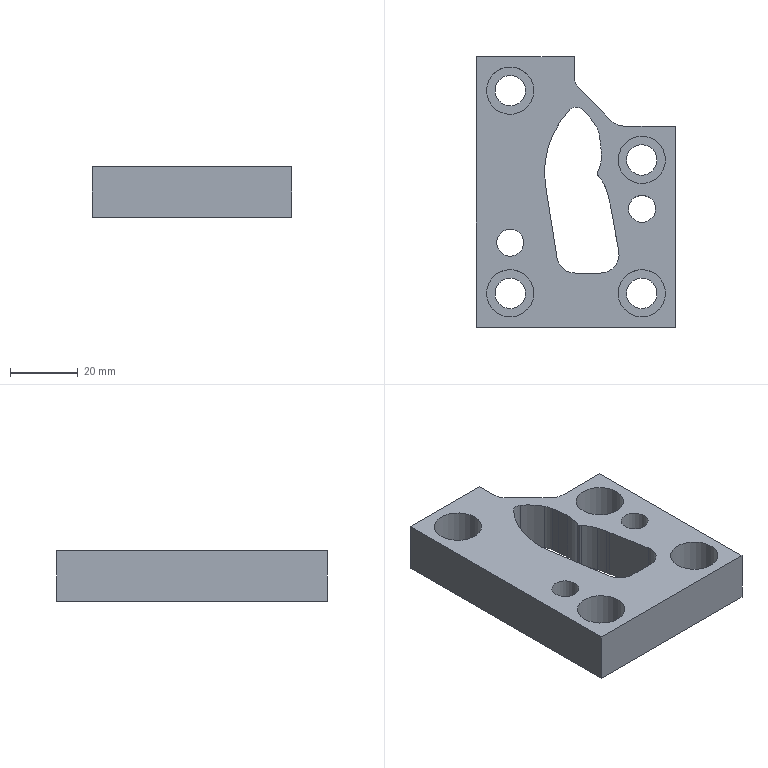Part | STEP file | 1 solid | 43 faces | box 58.914 x 80 x 15 mm | volume 42146 mm3 | cylinder 26 | plane 15 | spline 2 | commonest cylinder face diameters 9 x4 14 x4 8 x2 10 x2 11 x2 1.518 x1
STEP:
#1=CARTESIAN_POINT('',(-239.5,-87.5,-17.));
#2=VERTEX_POINT('',#1);
#3=CARTESIAN_POINT('',(-243.5,-87.5,-17.));
#4=DIRECTION('',(0.,0.,1.));
#5=DIRECTION('',(1.,0.,0.));
#6=AXIS2_PLACEMENT_3D('',#3,#4,#5);
#7=CIRCLE('',#6,4.);
#8=EDGE_CURVE('',#2,#2,#7,.T.);
#9=ORIENTED_EDGE('',*,*,#8,.T.);
#10=EDGE_LOOP('',(#9));
#11=FACE_BOUND('',#10,.T.);
#12=CARTESIAN_POINT('',(-278.5,-97.5,-17.));
#13=VERTEX_POINT('',#12);
#14=CARTESIAN_POINT('',(-282.5,-97.5,-17.));
#15=DIRECTION('',(0.,0.,1.));
#16=DIRECTION('',(1.,0.,0.));
#17=AXIS2_PLACEMENT_3D('',#14,#15,#16);
#18=CIRCLE('',#17,4.);
#19=EDGE_CURVE('',#13,#13,#18,.T.);
#20=ORIENTED_EDGE('',*,*,#19,.T.);
#21=EDGE_LOOP('',(#20));
#22=FACE_BOUND('',#21,.T.);
#23=CARTESIAN_POINT('',(-239.086,-73.,-17.));
#24=VERTEX_POINT('',#23);
#25=CARTESIAN_POINT('',(-243.586,-73.,-17.));
#26=DIRECTION('',(0.,0.,-1.));
#27=DIRECTION('',(1.,0.,0.));
#28=AXIS2_PLACEMENT_3D('',#25,#26,#27);
#29=CIRCLE('',#28,4.5);
#30=EDGE_CURVE('',#24,#24,#29,.T.);
#31=ORIENTED_EDGE('',*,*,#30,.F.);
#32=EDGE_LOOP('',(#31));
#33=FACE_BOUND('',#32,.T.);
#34=CARTESIAN_POINT('',(-287.,-112.5,-17.));
#35=VERTEX_POINT('',#34);
#36=CARTESIAN_POINT('',(-282.5,-112.5,-17.));
#37=DIRECTION('',(0.,0.,-1.));
#38=DIRECTION('',(-1.,0.,0.));
#39=AXIS2_PLACEMENT_3D('',#36,#37,#38);
#40=CIRCLE('',#39,4.5);
#41=EDGE_CURVE('',#35,#35,#40,.T.);
#42=ORIENTED_EDGE('',*,*,#41,.F.);
#43=EDGE_LOOP('',(#42));
#44=FACE_BOUND('',#43,.T.);
#45=CARTESIAN_POINT('',(-287.,-52.5,-17.));
#46=VERTEX_POINT('',#45);
#47=CARTESIAN_POINT('',(-282.5,-52.5,-17.));
#48=DIRECTION('',(0.,0.,1.));
#49=DIRECTION('',(-1.,0.,0.));
#50=AXIS2_PLACEMENT_3D('',#47,#48,#49);
#51=CIRCLE('',#50,4.5);
#52=EDGE_CURVE('',#46,#46,#51,.T.);
#53=ORIENTED_EDGE('',*,*,#52,.T.);
#54=EDGE_LOOP('',(#53));
#55=FACE_BOUND('',#54,.T.);
#56=CARTESIAN_POINT('',(-239.086,-112.5,-17.));
#57=VERTEX_POINT('',#56);
#58=CARTESIAN_POINT('',(-243.586,-112.5,-17.));
#59=DIRECTION('',(0.,0.,1.));
#60=DIRECTION('',(1.,0.,0.));
#61=AXIS2_PLACEMENT_3D('',#58,#59,#60);
#62=CIRCLE('',#61,4.5);
#63=EDGE_CURVE('',#57,#57,#62,.T.);
#64=ORIENTED_EDGE('',*,*,#63,.T.);
#65=EDGE_LOOP('',(#64));
#66=FACE_BOUND('',#65,.T.);
#67=CARTESIAN_POINT('',(-263.55,-48.378,-17.));
#68=VERTEX_POINT('',#67);
#69=CARTESIAN_POINT('',(-263.55,-42.5,-17.));
#70=VERTEX_POINT('',#69);
#71=CARTESIAN_POINT('',(-263.55,47.,-17.));
#72=DIRECTION('',(0.,1.,0.));
#73=VECTOR('',#72,1.);
#74=LINE('',#71,#73);
#75=EDGE_CURVE('',#68,#70,#74,.T.);
#76=ORIENTED_EDGE('',*,*,#75,.F.);
#77=CARTESIAN_POINT('',(-262.086,-51.914,-17.));
#78=VERTEX_POINT('',#77);
#79=CARTESIAN_POINT('',(-258.55,-48.378,-17.));
#80=DIRECTION('',(0.,0.,1.));
#81=DIRECTION('',(1.,0.,0.));
#82=AXIS2_PLACEMENT_3D('',#79,#80,#81);
#83=CIRCLE('',#82,5.);
#84=EDGE_CURVE('',#68,#78,#83,.T.);
#85=ORIENTED_EDGE('',*,*,#84,.T.);
#86=CARTESIAN_POINT('',(-252.464,-61.536,-17.));
#87=VERTEX_POINT('',#86);
#88=CARTESIAN_POINT('',(-203.505,-110.494,-17.));
#89=DIRECTION('',(0.7071,-0.7071,0.));
#90=VECTOR('',#89,1.);
#91=LINE('',#88,#90);
#92=EDGE_CURVE('',#78,#87,#91,.T.);
#93=ORIENTED_EDGE('',*,*,#92,.T.);
#94=CARTESIAN_POINT('',(-248.928,-63.,-17.));
#95=VERTEX_POINT('',#94);
#96=CARTESIAN_POINT('',(-248.928,-58.,-17.));
#97=DIRECTION('',(0.,0.,1.));
#98=DIRECTION('',(1.,0.,0.));
#99=AXIS2_PLACEMENT_3D('',#96,#97,#98);
#100=CIRCLE('',#99,5.);
#101=EDGE_CURVE('',#87,#95,#100,.T.);
#102=ORIENTED_EDGE('',*,*,#101,.T.);
#103=CARTESIAN_POINT('',(-233.586,-63.,-17.));
#104=VERTEX_POINT('',#103);
#105=CARTESIAN_POINT('',(-224.,-63.,-17.));
#106=DIRECTION('',(-1.,0.,0.));
#107=VECTOR('',#106,1.);
#108=LINE('',#105,#107);
#109=EDGE_CURVE('',#104,#95,#108,.T.);
#110=ORIENTED_EDGE('',*,*,#109,.F.);
#111=CARTESIAN_POINT('',(-233.586,-122.5,-17.));
#112=VERTEX_POINT('',#111);
#113=CARTESIAN_POINT('',(-233.586,-97.5,-17.));
#114=DIRECTION('',(0.,1.,0.));
#115=VECTOR('',#114,1.);
#116=LINE('',#113,#115);
#117=EDGE_CURVE('',#112,#104,#116,.T.);
#118=ORIENTED_EDGE('',*,*,#117,.F.);
#119=CARTESIAN_POINT('',(-292.5,-122.5,-17.));
#120=VERTEX_POINT('',#119);
#121=CARTESIAN_POINT('',(-262.5,-122.5,-17.));
#122=DIRECTION('',(1.,0.,0.));
#123=VECTOR('',#122,1.);
#124=LINE('',#121,#123);
#125=EDGE_CURVE('',#120,#112,#124,.T.);
#126=ORIENTED_EDGE('',*,*,#125,.F.);
#127=CARTESIAN_POINT('',(-292.5,-42.5,-17.));
#128=VERTEX_POINT('',#127);
#129=CARTESIAN_POINT('',(-292.5,49.2,-17.));
#130=DIRECTION('',(0.,1.,0.));
#131=VECTOR('',#130,1.);
#132=LINE('',#129,#131);
#133=EDGE_CURVE('',#120,#128,#132,.T.);
#134=ORIENTED_EDGE('',*,*,#133,.T.);
#135=CARTESIAN_POINT('',(-262.5,-42.5,-17.));
#136=DIRECTION('',(-1.,0.,0.));
#137=VECTOR('',#136,1.);
#138=LINE('',#135,#137);
#139=EDGE_CURVE('',#70,#128,#138,.T.);
#140=ORIENTED_EDGE('',*,*,#139,.F.);
#141=EDGE_LOOP('',(#76,#85,#93,#102,#110,#118,#126,#134,#140));
#142=FACE_BOUND('',#141,.T.);
#143=CARTESIAN_POINT('',(-250.392,-100.011,-17.));
#144=VERTEX_POINT('',#143);
#145=CARTESIAN_POINT('',(-255.802,-106.5,-17.));
#146=VERTEX_POINT('',#145);
#147=CARTESIAN_POINT('',(-255.802,-101.,-17.));
#148=DIRECTION('',(0.,0.,-1.));
#149=DIRECTION('',(1.,0.,0.));
#150=AXIS2_PLACEMENT_3D('',#147,#148,#149);
#151=CIRCLE('',#150,5.5);
#152=EDGE_CURVE('',#144,#146,#151,.T.);
#153=ORIENTED_EDGE('',*,*,#152,.F.);
#154=CARTESIAN_POINT('',(-252.857,-86.509,-17.));
#155=VERTEX_POINT('',#154);
#156=CARTESIAN_POINT('',(33298.208,6031.949,-17.));
#157=DIRECTION('',(0.,0.,-1.));
#158=DIRECTION('',(1.,0.,0.));
#159=AXIS2_PLACEMENT_3D('',#156,#157,#158);
#160=CIRCLE('',#159,34104.391);
#161=EDGE_CURVE('',#144,#155,#160,.T.);
#162=ORIENTED_EDGE('',*,*,#161,.T.);
#163=CARTESIAN_POINT('',(-253.088,-85.35,-17.));
#164=VERTEX_POINT('',#163);
#165=CARTESIAN_POINT('',(-289.905,-93.275,-17.));
#166=DIRECTION('',(0.,0.,1.));
#167=DIRECTION('',(1.,0.,0.));
#168=AXIS2_PLACEMENT_3D('',#165,#166,#167);
#169=CIRCLE('',#168,37.66);
#170=EDGE_CURVE('',#155,#164,#169,.T.);
#171=ORIENTED_EDGE('',*,*,#170,.T.);
#172=CARTESIAN_POINT('',(-253.879,-82.262,-17.));
#173=VERTEX_POINT('',#172);
#174=CARTESIAN_POINT('',(-292.811,-93.913,-17.));
#175=DIRECTION('',(0.,0.,1.));
#176=DIRECTION('',(1.,0.,0.));
#177=AXIS2_PLACEMENT_3D('',#174,#175,#176);
#178=CIRCLE('',#177,40.635);
#179=EDGE_CURVE('',#164,#173,#178,.T.);
#180=ORIENTED_EDGE('',*,*,#179,.T.);
#181=CARTESIAN_POINT('',(-256.293,-77.948,-17.));
#182=VERTEX_POINT('',#181);
#183=CARTESIAN_POINT('',(-264.943,-85.623,-17.));
#184=DIRECTION('',(0.,0.,1.));
#185=DIRECTION('',(1.,0.,0.));
#186=AXIS2_PLACEMENT_3D('',#183,#184,#185);
#187=CIRCLE('',#186,11.564);
#188=EDGE_CURVE('',#173,#182,#187,.T.);
#189=ORIENTED_EDGE('',*,*,#188,.T.);
#190=CARTESIAN_POINT('',(-256.599,-77.557,-17.));
#191=VERTEX_POINT('',#190);
#192=CARTESIAN_POINT('',(-252.81,-74.892,-17.));
#193=DIRECTION('',(0.,0.,-1.));
#194=DIRECTION('',(1.,0.,0.));
#195=AXIS2_PLACEMENT_3D('',#192,#193,#194);
#196=CIRCLE('',#195,4.634);
#197=EDGE_CURVE('',#182,#191,#196,.T.);
#198=ORIENTED_EDGE('',*,*,#197,.T.);
#199=CARTESIAN_POINT('',(-256.698,-76.822,-17.));
#200=VERTEX_POINT('',#199);
#201=CARTESIAN_POINT('',(-255.992,-77.101,-17.));
#202=DIRECTION('',(0.,0.,-1.));
#203=DIRECTION('',(1.,0.,0.));
#204=AXIS2_PLACEMENT_3D('',#201,#202,#203);
#205=CIRCLE('',#204,0.7592);
#206=EDGE_CURVE('',#191,#200,#205,.T.);
#207=ORIENTED_EDGE('',*,*,#206,.T.);
#208=CARTESIAN_POINT('',(-256.574,-76.515,-17.));
#209=VERTEX_POINT('',#208);
#210=CARTESIAN_POINT('',(-253.687,-77.89,-17.));
#211=DIRECTION('',(0.,0.,-1.));
#212=DIRECTION('',(1.,0.,0.));
#213=AXIS2_PLACEMENT_3D('',#210,#211,#212);
#214=CIRCLE('',#213,3.195);
#215=EDGE_CURVE('',#200,#209,#214,.T.);
#216=ORIENTED_EDGE('',*,*,#215,.T.);
#217=CARTESIAN_POINT('',(-255.525,-71.581,-17.));
#218=VERTEX_POINT('',#217);
#219=CARTESIAN_POINT('',(-266.229,-71.882,-17.));
#220=DIRECTION('',(0.,0.,1.));
#221=DIRECTION('',(1.,0.,0.));
#222=AXIS2_PLACEMENT_3D('',#219,#220,#221);
#223=CIRCLE('',#222,10.71);
#224=EDGE_CURVE('',#209,#218,#223,.T.);
#225=ORIENTED_EDGE('',*,*,#224,.T.);
#226=CARTESIAN_POINT('',(-255.83,-68.058,-17.));
#227=VERTEX_POINT('',#226);
#228=CARTESIAN_POINT('',(-288.806,-72.678,-17.));
#229=DIRECTION('',(0.,0.,1.));
#230=DIRECTION('',(1.,0.,0.));
#231=AXIS2_PLACEMENT_3D('',#228,#229,#230);
#232=CIRCLE('',#231,33.298);
#233=EDGE_CURVE('',#218,#227,#232,.T.);
#234=ORIENTED_EDGE('',*,*,#233,.T.);
#235=CARTESIAN_POINT('',(-256.146,-65.761,-17.));
#236=VERTEX_POINT('',#235);
#237=CARTESIAN_POINT('',(286.525,7.944,-17.));
#238=DIRECTION('',(0.,0.,-1.));
#239=DIRECTION('',(1.,0.,0.));
#240=AXIS2_PLACEMENT_3D('',#237,#238,#239);
#241=CIRCLE('',#240,547.653);
#242=EDGE_CURVE('',#227,#236,#241,.T.);
#243=ORIENTED_EDGE('',*,*,#242,.T.);
#244=CARTESIAN_POINT('',(-257.012,-63.252,-17.));
#245=VERTEX_POINT('',#244);
#246=CARTESIAN_POINT('',(-262.853,-66.672,-17.));
#247=DIRECTION('',(0.,0.,1.));
#248=DIRECTION('',(1.,0.,0.));
#249=AXIS2_PLACEMENT_3D('',#246,#247,#248);
#250=CIRCLE('',#249,6.768);
#251=EDGE_CURVE('',#236,#245,#250,.T.);
#252=ORIENTED_EDGE('',*,*,#251,.T.);
#253=CARTESIAN_POINT('',(-261.559,-57.918,-17.));
#254=VERTEX_POINT('',#253);
#255=CARTESIAN_POINT('',(-257.012,-63.252,-17.));
#256=CARTESIAN_POINT('',(-258.204,-61.218,-17.));
#257=CARTESIAN_POINT('',(-259.658,-59.325,-17.));
#258=CARTESIAN_POINT('',(-261.559,-57.918,-17.));
#259=B_SPLINE_CURVE_WITH_KNOTS('',3,(#255,#256,#257,#258),.UNSPECIFIED.,.F.,.F.,(4,4),(0.,1.),.UNSPECIFIED.);
#260=EDGE_CURVE('',#245,#254,#259,.T.);
#261=ORIENTED_EDGE('',*,*,#260,.T.);
#262=CARTESIAN_POINT('',(-264.842,-58.187,-17.));
#263=VERTEX_POINT('',#262);
#264=CARTESIAN_POINT('',(-263.047,-59.927,-17.));
#265=DIRECTION('',(0.,0.,-1.));
#266=DIRECTION('',(1.,0.,0.));
#267=AXIS2_PLACEMENT_3D('',#264,#265,#266);
#268=CIRCLE('',#267,2.5);
#269=EDGE_CURVE('',#263,#254,#268,.T.);
#270=ORIENTED_EDGE('',*,*,#269,.F.);
#271=CARTESIAN_POINT('',(-271.999,-80.759,-17.));
#272=VERTEX_POINT('',#271);
#273=CARTESIAN_POINT('',(-264.842,-58.187,-17.));
#274=CARTESIAN_POINT('',(-266.278,-59.668,-17.));
#275=CARTESIAN_POINT('',(-267.514,-61.287,-17.));
#276=CARTESIAN_POINT('',(-269.608,-64.784,-17.));
#277=CARTESIAN_POINT('',(-270.466,-66.681,-17.));
#278=CARTESIAN_POINT('',(-272.311,-72.501,-17.));
#279=CARTESIAN_POINT('',(-272.635,-76.684,-17.));
#280=CARTESIAN_POINT('',(-271.999,-80.759,-17.));
#281=B_SPLINE_CURVE_WITH_KNOTS('',3,(#273,#274,#275,#276,#277,#278,#279,#280),.UNSPECIFIED.,.F.,.F.,(4,2,2,4),(0.,0.25,0.5,1.),.UNSPECIFIED.);
#282=EDGE_CURVE('',#263,#272,#281,.T.);
#283=ORIENTED_EDGE('',*,*,#282,.T.);
#284=CARTESIAN_POINT('',(-268.678,-101.855,-17.));
#285=VERTEX_POINT('',#284);
#286=CARTESIAN_POINT('',(-286.444,11.004,-17.));
#287=DIRECTION('',(0.1555,-0.9878,0.));
#288=VECTOR('',#287,1.);
#289=LINE('',#286,#288);
#290=EDGE_CURVE('',#272,#285,#289,.T.);
#291=ORIENTED_EDGE('',*,*,#290,.T.);
#292=CARTESIAN_POINT('',(-263.245,-106.5,-17.));
#293=VERTEX_POINT('',#292);
#294=CARTESIAN_POINT('',(-263.245,-101.,-17.));
#295=DIRECTION('',(0.,0.,-1.));
#296=DIRECTION('',(1.,0.,0.));
#297=AXIS2_PLACEMENT_3D('',#294,#295,#296);
#298=CIRCLE('',#297,5.5);
#299=EDGE_CURVE('',#293,#285,#298,.T.);
#300=ORIENTED_EDGE('',*,*,#299,.F.);
#301=CARTESIAN_POINT('',(-43.811,-106.5,-17.));
#302=DIRECTION('',(-1.,0.,0.));
#303=VECTOR('',#302,1.);
#304=LINE('',#301,#303);
#305=EDGE_CURVE('',#146,#293,#304,.T.);
#306=ORIENTED_EDGE('',*,*,#305,.F.);
#307=EDGE_LOOP('',(#153,#162,#171,#180,#189,#198,#207,#216,#225,#234,#243,#252,#261,#270,#283,#291,#300,#306));
#308=FACE_BOUND('',#307,.T.);
#309=CARTESIAN_POINT('',(-43.811,49.2,-17.));
#310=DIRECTION('',(0.,0.,1.));
#311=DIRECTION('',(1.,0.,0.));
#312=AXIS2_PLACEMENT_3D('',#309,#310,#311);
#313=PLANE('',#312);
#314=ADVANCED_FACE('',(#11,#22,#33,#44,#55,#66,#142,#308),#313,.F.);
#315=CARTESIAN_POINT('',(-239.5,-87.5,-2.));
#316=VERTEX_POINT('',#315);
#317=CARTESIAN_POINT('',(-243.5,-87.5,-2.));
#318=DIRECTION('',(0.,0.,-1.));
#319=DIRECTION('',(1.,0.,0.));
#320=AXIS2_PLACEMENT_3D('',#317,#318,#319);
#321=CIRCLE('',#320,4.);
#322=EDGE_CURVE('',#316,#316,#321,.T.);
#323=ORIENTED_EDGE('',*,*,#322,.T.);
#324=EDGE_LOOP('',(#323));
#325=FACE_BOUND('',#324,.T.);
#326=CARTESIAN_POINT('',(-278.5,-97.5,-2.));
#327=VERTEX_POINT('',#326);
#328=CARTESIAN_POINT('',(-282.5,-97.5,-2.));
#329=DIRECTION('',(0.,0.,-1.));
#330=DIRECTION('',(1.,0.,0.));
#331=AXIS2_PLACEMENT_3D('',#328,#329,#330);
#332=CIRCLE('',#331,4.);
#333=EDGE_CURVE('',#327,#327,#332,.T.);
#334=ORIENTED_EDGE('',*,*,#333,.T.);
#335=EDGE_LOOP('',(#334));
#336=FACE_BOUND('',#335,.T.);
#337=CARTESIAN_POINT('',(-236.586,-73.,-2.));
#338=VERTEX_POINT('',#337);
#339=CARTESIAN_POINT('',(-243.586,-73.,-2.));
#340=DIRECTION('',(0.,0.,1.));
#341=DIRECTION('',(1.,0.,0.));
#342=AXIS2_PLACEMENT_3D('',#339,#340,#341);
#343=CIRCLE('',#342,7.);
#344=EDGE_CURVE('',#338,#338,#343,.T.);
#345=ORIENTED_EDGE('',*,*,#344,.F.);
#346=EDGE_LOOP('',(#345));
#347=FACE_BOUND('',#346,.T.);
#348=CARTESIAN_POINT('',(-289.5,-112.5,-2.));
#349=VERTEX_POINT('',#348);
#350=CARTESIAN_POINT('',(-282.5,-112.5,-2.));
#351=DIRECTION('',(0.,0.,1.));
#352=DIRECTION('',(-1.,0.,0.));
#353=AXIS2_PLACEMENT_3D('',#350,#351,#352);
#354=CIRCLE('',#353,7.);
#355=EDGE_CURVE('',#349,#349,#354,.T.);
#356=ORIENTED_EDGE('',*,*,#355,.F.);
#357=EDGE_LOOP('',(#356));
#358=FACE_BOUND('',#357,.T.);
#359=CARTESIAN_POINT('',(-289.5,-52.5,-2.));
#360=VERTEX_POINT('',#359);
#361=CARTESIAN_POINT('',(-282.5,-52.5,-2.));
#362=DIRECTION('',(0.,0.,-1.));
#363=DIRECTION('',(-1.,0.,0.));
#364=AXIS2_PLACEMENT_3D('',#361,#362,#363);
#365=CIRCLE('',#364,7.);
#366=EDGE_CURVE('',#360,#360,#365,.T.);
#367=ORIENTED_EDGE('',*,*,#366,.T.);
#368=EDGE_LOOP('',(#367));
#369=FACE_BOUND('',#368,.T.);
#370=CARTESIAN_POINT('',(-236.586,-112.5,-2.));
#371=VERTEX_POINT('',#370);
#372=CARTESIAN_POINT('',(-243.586,-112.5,-2.));
#373=DIRECTION('',(0.,0.,-1.));
#374=DIRECTION('',(1.,0.,0.));
#375=AXIS2_PLACEMENT_3D('',#372,#373,#374);
#376=CIRCLE('',#375,7.);
#377=EDGE_CURVE('',#371,#371,#376,.T.);
#378=ORIENTED_EDGE('',*,*,#377,.T.);
#379=EDGE_LOOP('',(#378));
#380=FACE_BOUND('',#379,.T.);
#381=CARTESIAN_POINT('',(-262.086,-51.914,-2.));
#382=VERTEX_POINT('',#381);
#383=CARTESIAN_POINT('',(-252.464,-61.536,-2.));
#384=VERTEX_POINT('',#383);
#385=CARTESIAN_POINT('',(-203.505,-110.494,-2.));
#386=DIRECTION('',(0.7071,-0.7071,0.));
#387=VECTOR('',#386,1.);
#388=LINE('',#385,#387);
#389=EDGE_CURVE('',#382,#384,#388,.T.);
#390=ORIENTED_EDGE('',*,*,#389,.F.);
#391=CARTESIAN_POINT('',(-263.55,-48.378,-2.));
#392=VERTEX_POINT('',#391);
#393=CARTESIAN_POINT('',(-258.55,-48.378,-2.));
#394=DIRECTION('',(0.,0.,-1.));
#395=DIRECTION('',(1.,0.,0.));
#396=AXIS2_PLACEMENT_3D('',#393,#394,#395);
#397=CIRCLE('',#396,5.);
#398=EDGE_CURVE('',#382,#392,#397,.T.);
#399=ORIENTED_EDGE('',*,*,#398,.T.);
#400=CARTESIAN_POINT('',(-263.55,-42.5,-2.));
#401=VERTEX_POINT('',#400);
#402=CARTESIAN_POINT('',(-263.55,47.,-2.));
#403=DIRECTION('',(0.,1.,0.));
#404=VECTOR('',#403,1.);
#405=LINE('',#402,#404);
#406=EDGE_CURVE('',#392,#401,#405,.T.);
#407=ORIENTED_EDGE('',*,*,#406,.T.);
#408=CARTESIAN_POINT('',(-292.5,-42.5,-2.));
#409=VERTEX_POINT('',#408);
#410=CARTESIAN_POINT('',(-262.5,-42.5,-2.));
#411=DIRECTION('',(-1.,0.,0.));
#412=VECTOR('',#411,1.);
#413=LINE('',#410,#412);
#414=EDGE_CURVE('',#401,#409,#413,.T.);
#415=ORIENTED_EDGE('',*,*,#414,.T.);
#416=CARTESIAN_POINT('',(-292.5,-122.5,-2.));
#417=VERTEX_POINT('',#416);
#418=CARTESIAN_POINT('',(-292.5,49.2,-2.));
#419=DIRECTION('',(0.,1.,0.));
#420=VECTOR('',#419,1.);
#421=LINE('',#418,#420);
#422=EDGE_CURVE('',#417,#409,#421,.T.);
#423=ORIENTED_EDGE('',*,*,#422,.F.);
#424=CARTESIAN_POINT('',(-233.586,-122.5,-2.));
#425=VERTEX_POINT('',#424);
#426=CARTESIAN_POINT('',(-262.5,-122.5,-2.));
#427=DIRECTION('',(1.,0.,0.));
#428=VECTOR('',#427,1.);
#429=LINE('',#426,#428);
#430=EDGE_CURVE('',#417,#425,#429,.T.);
#431=ORIENTED_EDGE('',*,*,#430,.T.);
#432=CARTESIAN_POINT('',(-233.586,-63.,-2.));
#433=VERTEX_POINT('',#432);
#434=CARTESIAN_POINT('',(-233.586,-97.5,-2.));
#435=DIRECTION('',(0.,1.,0.));
#436=VECTOR('',#435,1.);
#437=LINE('',#434,#436);
#438=EDGE_CURVE('',#425,#433,#437,.T.);
#439=ORIENTED_EDGE('',*,*,#438,.T.);
#440=CARTESIAN_POINT('',(-248.928,-63.,-2.));
#441=VERTEX_POINT('',#440);
#442=CARTESIAN_POINT('',(-224.,-63.,-2.));
#443=DIRECTION('',(-1.,0.,0.));
#444=VECTOR('',#443,1.);
#445=LINE('',#442,#444);
#446=EDGE_CURVE('',#433,#441,#445,.T.);
#447=ORIENTED_EDGE('',*,*,#446,.T.);
#448=CARTESIAN_POINT('',(-248.928,-58.,-2.));
#449=DIRECTION('',(0.,0.,-1.));
#450=DIRECTION('',(1.,0.,0.));
#451=AXIS2_PLACEMENT_3D('',#448,#449,#450);
#452=CIRCLE('',#451,5.);
#453=EDGE_CURVE('',#441,#384,#452,.T.);
#454=ORIENTED_EDGE('',*,*,#453,.T.);
#455=EDGE_LOOP('',(#390,#399,#407,#415,#423,#431,#439,#447,#454));
#456=FACE_BOUND('',#455,.T.);
#457=CARTESIAN_POINT('',(-257.012,-63.252,-2.));
#458=VERTEX_POINT('',#457);
#459=CARTESIAN_POINT('',(-261.559,-57.918,-2.));
#460=VERTEX_POINT('',#459);
#461=CARTESIAN_POINT('',(-257.012,-63.252,-2.));
#462=CARTESIAN_POINT('',(-258.204,-61.218,-2.));
#463=CARTESIAN_POINT('',(-259.658,-59.325,-2.));
#464=CARTESIAN_POINT('',(-261.559,-57.918,-2.));
#465=B_SPLINE_CURVE_WITH_KNOTS('',3,(#461,#462,#463,#464),.UNSPECIFIED.,.F.,.F.,(4,4),(0.,1.),.UNSPECIFIED.);
#466=EDGE_CURVE('',#458,#460,#465,.T.);
#467=ORIENTED_EDGE('',*,*,#466,.F.);
#468=CARTESIAN_POINT('',(-256.146,-65.761,-2.));
#469=VERTEX_POINT('',#468);
#470=CARTESIAN_POINT('',(-262.853,-66.672,-2.));
#471=DIRECTION('',(0.,0.,1.));
#472=DIRECTION('',(1.,0.,0.));
#473=AXIS2_PLACEMENT_3D('',#470,#471,#472);
#474=CIRCLE('',#473,6.768);
#475=EDGE_CURVE('',#469,#458,#474,.T.);
#476=ORIENTED_EDGE('',*,*,#475,.F.);
#477=CARTESIAN_POINT('',(-255.83,-68.058,-2.));
#478=VERTEX_POINT('',#477);
#479=CARTESIAN_POINT('',(286.525,7.944,-2.));
#480=DIRECTION('',(0.,0.,-1.));
#481=DIRECTION('',(1.,0.,0.));
#482=AXIS2_PLACEMENT_3D('',#479,#480,#481);
#483=CIRCLE('',#482,547.653);
#484=EDGE_CURVE('',#478,#469,#483,.T.);
#485=ORIENTED_EDGE('',*,*,#484,.F.);
#486=CARTESIAN_POINT('',(-255.525,-71.581,-2.));
#487=VERTEX_POINT('',#486);
#488=CARTESIAN_POINT('',(-288.806,-72.678,-2.));
#489=DIRECTION('',(0.,0.,1.));
#490=DIRECTION('',(1.,0.,0.));
#491=AXIS2_PLACEMENT_3D('',#488,#489,#490);
#492=CIRCLE('',#491,33.298);
#493=EDGE_CURVE('',#487,#478,#492,.T.);
#494=ORIENTED_EDGE('',*,*,#493,.F.);
#495=CARTESIAN_POINT('',(-256.574,-76.515,-2.));
#496=VERTEX_POINT('',#495);
#497=CARTESIAN_POINT('',(-266.229,-71.882,-2.));
#498=DIRECTION('',(0.,0.,1.));
#499=DIRECTION('',(1.,0.,0.));
#500=AXIS2_PLACEMENT_3D('',#497,#498,#499);
#501=CIRCLE('',#500,10.71);
#502=EDGE_CURVE('',#496,#487,#501,.T.);
#503=ORIENTED_EDGE('',*,*,#502,.F.);
#504=CARTESIAN_POINT('',(-256.698,-76.822,-2.));
#505=VERTEX_POINT('',#504);
#506=CARTESIAN_POINT('',(-253.687,-77.89,-2.));
#507=DIRECTION('',(0.,0.,1.));
#508=DIRECTION('',(1.,0.,0.));
#509=AXIS2_PLACEMENT_3D('',#506,#507,#508);
#510=CIRCLE('',#509,3.195);
#511=EDGE_CURVE('',#496,#505,#510,.T.);
#512=ORIENTED_EDGE('',*,*,#511,.T.);
#513=CARTESIAN_POINT('',(-256.599,-77.557,-2.));
#514=VERTEX_POINT('',#513);
#515=CARTESIAN_POINT('',(-255.992,-77.101,-2.));
#516=DIRECTION('',(0.,0.,-1.));
#517=DIRECTION('',(1.,0.,0.));
#518=AXIS2_PLACEMENT_3D('',#515,#516,#517);
#519=CIRCLE('',#518,0.7592);
#520=EDGE_CURVE('',#514,#505,#519,.T.);
#521=ORIENTED_EDGE('',*,*,#520,.F.);
#522=CARTESIAN_POINT('',(-256.293,-77.948,-2.));
#523=VERTEX_POINT('',#522);
#524=CARTESIAN_POINT('',(-252.81,-74.892,-2.));
#525=DIRECTION('',(0.,0.,1.));
#526=DIRECTION('',(1.,0.,0.));
#527=AXIS2_PLACEMENT_3D('',#524,#525,#526);
#528=CIRCLE('',#527,4.634);
#529=EDGE_CURVE('',#514,#523,#528,.T.);
#530=ORIENTED_EDGE('',*,*,#529,.T.);
#531=CARTESIAN_POINT('',(-253.879,-82.262,-2.));
#532=VERTEX_POINT('',#531);
#533=CARTESIAN_POINT('',(-264.943,-85.623,-2.));
#534=DIRECTION('',(0.,0.,-1.));
#535=DIRECTION('',(1.,0.,0.));
#536=AXIS2_PLACEMENT_3D('',#533,#534,#535);
#537=CIRCLE('',#536,11.564);
#538=EDGE_CURVE('',#523,#532,#537,.T.);
#539=ORIENTED_EDGE('',*,*,#538,.T.);
#540=CARTESIAN_POINT('',(-253.088,-85.35,-2.));
#541=VERTEX_POINT('',#540);
#542=CARTESIAN_POINT('',(-292.811,-93.913,-2.));
#543=DIRECTION('',(0.,0.,-1.));
#544=DIRECTION('',(1.,0.,0.));
#545=AXIS2_PLACEMENT_3D('',#542,#543,#544);
#546=CIRCLE('',#545,40.635);
#547=EDGE_CURVE('',#532,#541,#546,.T.);
#548=ORIENTED_EDGE('',*,*,#547,.T.);
#549=CARTESIAN_POINT('',(-252.857,-86.509,-2.));
#550=VERTEX_POINT('',#549);
#551=CARTESIAN_POINT('',(-289.905,-93.275,-2.));
#552=DIRECTION('',(0.,0.,-1.));
#553=DIRECTION('',(1.,0.,0.));
#554=AXIS2_PLACEMENT_3D('',#551,#552,#553);
#555=CIRCLE('',#554,37.66);
#556=EDGE_CURVE('',#541,#550,#555,.T.);
#557=ORIENTED_EDGE('',*,*,#556,.T.);
#558=CARTESIAN_POINT('',(-250.392,-100.011,-2.));
#559=VERTEX_POINT('',#558);
#560=CARTESIAN_POINT('',(33298.208,6031.949,-2.));
#561=DIRECTION('',(0.,0.,1.));
#562=DIRECTION('',(1.,0.,0.));
#563=AXIS2_PLACEMENT_3D('',#560,#561,#562);
#564=CIRCLE('',#563,34104.391);
#565=EDGE_CURVE('',#550,#559,#564,.T.);
#566=ORIENTED_EDGE('',*,*,#565,.T.);
#567=CARTESIAN_POINT('',(-255.802,-106.5,-2.));
#568=VERTEX_POINT('',#567);
#569=CARTESIAN_POINT('',(-255.802,-101.,-2.));
#570=DIRECTION('',(0.,0.,-1.));
#571=DIRECTION('',(1.,0.,0.));
#572=AXIS2_PLACEMENT_3D('',#569,#570,#571);
#573=CIRCLE('',#572,5.5);
#574=EDGE_CURVE('',#559,#568,#573,.T.);
#575=ORIENTED_EDGE('',*,*,#574,.T.);
#576=CARTESIAN_POINT('',(-263.245,-106.5,-2.));
#577=VERTEX_POINT('',#576);
#578=CARTESIAN_POINT('',(-43.811,-106.5,-2.));
#579=DIRECTION('',(-1.,0.,0.));
#580=VECTOR('',#579,1.);
#581=LINE('',#578,#580);
#582=EDGE_CURVE('',#568,#577,#581,.T.);
#583=ORIENTED_EDGE('',*,*,#582,.T.);
#584=CARTESIAN_POINT('',(-268.678,-101.855,-2.));
#585=VERTEX_POINT('',#584);
#586=CARTESIAN_POINT('',(-263.245,-101.,-2.));
#587=DIRECTION('',(0.,0.,-1.));
#588=DIRECTION('',(1.,0.,0.));
#589=AXIS2_PLACEMENT_3D('',#586,#587,#588);
#590=CIRCLE('',#589,5.5);
#591=EDGE_CURVE('',#577,#585,#590,.T.);
#592=ORIENTED_EDGE('',*,*,#591,.T.);
#593=CARTESIAN_POINT('',(-271.999,-80.759,-2.));
#594=VERTEX_POINT('',#593);
#595=CARTESIAN_POINT('',(-268.146,-105.233,-2.));
#596=DIRECTION('',(-0.1555,0.9878,0.));
#597=VECTOR('',#596,1.);
#598=LINE('',#595,#597);
#599=EDGE_CURVE('',#585,#594,#598,.T.);
#600=ORIENTED_EDGE('',*,*,#599,.T.);
#601=CARTESIAN_POINT('',(-264.842,-58.187,-2.));
#602=VERTEX_POINT('',#601);
#603=CARTESIAN_POINT('',(-264.842,-58.187,-2.));
#604=CARTESIAN_POINT('',(-266.278,-59.668,-2.));
#605=CARTESIAN_POINT('',(-267.514,-61.287,-2.));
#606=CARTESIAN_POINT('',(-269.608,-64.784,-2.));
#607=CARTESIAN_POINT('',(-270.466,-66.681,-2.));
#608=CARTESIAN_POINT('',(-272.311,-72.501,-2.));
#609=CARTESIAN_POINT('',(-272.635,-76.684,-2.));
#610=CARTESIAN_POINT('',(-271.999,-80.759,-2.));
#611=B_SPLINE_CURVE_WITH_KNOTS('',3,(#603,#604,#605,#606,#607,#608,#609,#610),.UNSPECIFIED.,.F.,.F.,(4,2,2,4),(0.,0.25,0.5,1.),.UNSPECIFIED.);
#612=EDGE_CURVE('',#602,#594,#611,.T.);
#613=ORIENTED_EDGE('',*,*,#612,.F.);
#614=CARTESIAN_POINT('',(-263.047,-59.927,-2.));
#615=DIRECTION('',(0.,0.,1.));
#616=DIRECTION('',(1.,0.,0.));
#617=AXIS2_PLACEMENT_3D('',#614,#615,#616);
#618=CIRCLE('',#617,2.5);
#619=EDGE_CURVE('',#460,#602,#618,.T.);
#620=ORIENTED_EDGE('',*,*,#619,.F.);
#621=EDGE_LOOP('',(#467,#476,#485,#494,#503,#512,#521,#530,#539,#548,#557,#566,#575,#583,#592,#600,#613,#620));
#622=FACE_BOUND('',#621,.T.);
#623=CARTESIAN_POINT('',(-43.811,49.2,-2.));
#624=DIRECTION('',(0.,0.,1.));
#625=DIRECTION('',(1.,0.,0.));
#626=AXIS2_PLACEMENT_3D('',#623,#624,#625);
#627=PLANE('',#626);
#628=ADVANCED_FACE('',(#325,#336,#347,#358,#369,#380,#456,#622),#627,.T.);
#629=CARTESIAN_POINT('',(-233.586,-63.,-2.));
#630=DIRECTION('',(0.,0.,-1.));
#631=VECTOR('',#630,1.);
#632=LINE('',#629,#631);
#633=EDGE_CURVE('',#433,#104,#632,.T.);
#634=ORIENTED_EDGE('',*,*,#633,.F.);
#635=ORIENTED_EDGE('',*,*,#438,.F.);
#636=CARTESIAN_POINT('',(-233.586,-122.5,-2.));
#637=DIRECTION('',(0.,0.,-1.));
#638=VECTOR('',#637,1.);
#639=LINE('',#636,#638);
#640=EDGE_CURVE('',#425,#112,#639,.T.);
#641=ORIENTED_EDGE('',*,*,#640,.T.);
#642=ORIENTED_EDGE('',*,*,#117,.T.);
#643=EDGE_LOOP('',(#634,#635,#641,#642));
#644=FACE_OUTER_BOUND('',#643,.T.);
#645=CARTESIAN_POINT('',(-233.586,-97.5,-2.));
#646=DIRECTION('',(1.,0.,0.));
#647=DIRECTION('',(0.,1.,0.));
#648=AXIS2_PLACEMENT_3D('',#645,#646,#647);
#649=PLANE('',#648);
#650=ADVANCED_FACE('',(#644),#649,.T.);
#651=ORIENTED_EDGE('',*,*,#640,.F.);
#652=ORIENTED_EDGE('',*,*,#430,.F.);
#653=CARTESIAN_POINT('',(-292.5,-122.5,-47.));
#654=DIRECTION('',(0.,0.,-1.));
#655=VECTOR('',#654,1.);
#656=LINE('',#653,#655);
#657=EDGE_CURVE('',#417,#120,#656,.T.);
#658=ORIENTED_EDGE('',*,*,#657,.T.);
#659=ORIENTED_EDGE('',*,*,#125,.T.);
#660=EDGE_LOOP('',(#651,#652,#658,#659));
#661=FACE_OUTER_BOUND('',#660,.T.);
#662=CARTESIAN_POINT('',(-262.5,-122.5,-47.));
#663=DIRECTION('',(0.,1.,0.));
#664=DIRECTION('',(1.,0.,0.));
#665=AXIS2_PLACEMENT_3D('',#662,#663,#664);
#666=PLANE('',#665);
#667=ADVANCED_FACE('',(#661),#666,.F.);
#668=ORIENTED_EDGE('',*,*,#657,.F.);
#669=ORIENTED_EDGE('',*,*,#422,.T.);
#670=CARTESIAN_POINT('',(-292.5,-42.5,-47.));
#671=DIRECTION('',(0.,0.,-1.));
#672=VECTOR('',#671,1.);
#673=LINE('',#670,#672);
#674=EDGE_CURVE('',#409,#128,#673,.T.);
#675=ORIENTED_EDGE('',*,*,#674,.T.);
#676=ORIENTED_EDGE('',*,*,#133,.F.);
#677=EDGE_LOOP('',(#668,#669,#675,#676));
#678=FACE_OUTER_BOUND('',#677,.T.);
#679=CARTESIAN_POINT('',(-292.5,0.,-47.));
#680=DIRECTION('',(1.,0.,0.));
#681=DIRECTION('',(0.,-1.,0.));
#682=AXIS2_PLACEMENT_3D('',#679,#680,#681);
#683=PLANE('',#682);
#684=ADVANCED_FACE('',(#678),#683,.F.);
#685=ORIENTED_EDGE('',*,*,#674,.F.);
#686=ORIENTED_EDGE('',*,*,#414,.F.);
#687=CARTESIAN_POINT('',(-263.55,-42.5,-47.));
#688=DIRECTION('',(0.,0.,-1.));
#689=VECTOR('',#688,1.);
#690=LINE('',#687,#689);
#691=EDGE_CURVE('',#401,#70,#690,.T.);
#692=ORIENTED_EDGE('',*,*,#691,.T.);
#693=ORIENTED_EDGE('',*,*,#139,.T.);
#694=EDGE_LOOP('',(#685,#686,#692,#693));
#695=FACE_OUTER_BOUND('',#694,.T.);
#696=CARTESIAN_POINT('',(-262.5,-42.5,-47.));
#697=DIRECTION('',(0.,-1.,0.));
#698=DIRECTION('',(-1.,0.,0.));
#699=AXIS2_PLACEMENT_3D('',#696,#697,#698);
#700=PLANE('',#699);
#701=ADVANCED_FACE('',(#695),#700,.F.);
#702=ORIENTED_EDGE('',*,*,#406,.F.);
#703=CARTESIAN_POINT('',(-263.55,-48.378,-17.));
#704=DIRECTION('',(0.,0.,-1.));
#705=VECTOR('',#704,1.);
#706=LINE('',#703,#705);
#707=EDGE_CURVE('',#392,#68,#706,.T.);
#708=ORIENTED_EDGE('',*,*,#707,.T.);
#709=ORIENTED_EDGE('',*,*,#75,.T.);
#710=ORIENTED_EDGE('',*,*,#691,.F.);
#711=EDGE_LOOP('',(#702,#708,#709,#710));
#712=FACE_OUTER_BOUND('',#711,.T.);
#713=CARTESIAN_POINT('',(-263.55,47.,-2.));
#714=DIRECTION('',(1.,0.,0.));
#715=DIRECTION('',(0.,1.,0.));
#716=AXIS2_PLACEMENT_3D('',#713,#714,#715);
#717=PLANE('',#716);
#718=ADVANCED_FACE('',(#712),#717,.T.);
#719=ORIENTED_EDGE('',*,*,#389,.T.);
#720=CARTESIAN_POINT('',(-252.464,-61.536,-17.));
#721=DIRECTION('',(0.,0.,-1.));
#722=VECTOR('',#721,1.);
#723=LINE('',#720,#722);
#724=EDGE_CURVE('',#384,#87,#723,.T.);
#725=ORIENTED_EDGE('',*,*,#724,.T.);
#726=ORIENTED_EDGE('',*,*,#92,.F.);
#727=CARTESIAN_POINT('',(-262.086,-51.914,-2.));
#728=DIRECTION('',(0.,0.,1.));
#729=VECTOR('',#728,1.);
#730=LINE('',#727,#729);
#731=EDGE_CURVE('',#78,#382,#730,.T.);
#732=ORIENTED_EDGE('',*,*,#731,.T.);
#733=EDGE_LOOP('',(#719,#725,#726,#732));
#734=FACE_OUTER_BOUND('',#733,.T.);
#735=CARTESIAN_POINT('',(-259.5,-54.5,-30.));
#736=DIRECTION('',(0.7071,0.7071,0.));
#737=DIRECTION('',(0.,0.,1.));
#738=AXIS2_PLACEMENT_3D('',#735,#736,#737);
#739=PLANE('',#738);
#740=ADVANCED_FACE('',(#734),#739,.T.);
#741=ORIENTED_EDGE('',*,*,#109,.T.);
#742=CARTESIAN_POINT('',(-248.928,-63.,-2.));
#743=DIRECTION('',(0.,0.,1.));
#744=VECTOR('',#743,1.);
#745=LINE('',#742,#744);
#746=EDGE_CURVE('',#95,#441,#745,.T.);
#747=ORIENTED_EDGE('',*,*,#746,.T.);
#748=ORIENTED_EDGE('',*,*,#446,.F.);
#749=ORIENTED_EDGE('',*,*,#633,.T.);
#750=EDGE_LOOP('',(#741,#747,#748,#749));
#751=FACE_OUTER_BOUND('',#750,.T.);
#752=CARTESIAN_POINT('',(-224.,-63.,-2.));
#753=DIRECTION('',(0.,1.,0.));
#754=DIRECTION('',(-1.,0.,0.));
#755=AXIS2_PLACEMENT_3D('',#752,#753,#754);
#756=PLANE('',#755);
#757=ADVANCED_FACE('',(#751),#756,.T.);
#758=ORIENTED_EDGE('',*,*,#453,.F.);
#759=ORIENTED_EDGE('',*,*,#746,.F.);
#760=ORIENTED_EDGE('',*,*,#101,.F.);
#761=ORIENTED_EDGE('',*,*,#724,.F.);
#762=EDGE_LOOP('',(#758,#759,#760,#761));
#763=FACE_OUTER_BOUND('',#762,.T.);
#764=CARTESIAN_POINT('',(-248.928,-58.,-30.));
#765=DIRECTION('',(0.,0.,1.));
#766=DIRECTION('',(1.,0.,0.));
#767=AXIS2_PLACEMENT_3D('',#764,#765,#766);
#768=CYLINDRICAL_SURFACE('',#767,5.);
#769=ADVANCED_FACE('',(#763),#768,.F.);
#770=ORIENTED_EDGE('',*,*,#398,.F.);
#771=ORIENTED_EDGE('',*,*,#731,.F.);
#772=ORIENTED_EDGE('',*,*,#84,.F.);
#773=ORIENTED_EDGE('',*,*,#707,.F.);
#774=EDGE_LOOP('',(#770,#771,#772,#773));
#775=FACE_OUTER_BOUND('',#774,.T.);
#776=CARTESIAN_POINT('',(-258.55,-48.378,-2.));
#777=DIRECTION('',(0.,0.,1.));
#778=DIRECTION('',(1.,0.,0.));
#779=AXIS2_PLACEMENT_3D('',#776,#777,#778);
#780=CYLINDRICAL_SURFACE('',#779,5.);
#781=ADVANCED_FACE('',(#775),#780,.F.);
#782=ORIENTED_EDGE('',*,*,#305,.T.);
#783=CARTESIAN_POINT('',(-263.245,-106.5,-185.));
#784=DIRECTION('',(0.,0.,1.));
#785=VECTOR('',#784,1.);
#786=LINE('',#783,#785);
#787=EDGE_CURVE('',#293,#577,#786,.T.);
#788=ORIENTED_EDGE('',*,*,#787,.T.);
#789=ORIENTED_EDGE('',*,*,#582,.F.);
#790=CARTESIAN_POINT('',(-255.802,-106.5,-185.));
#791=DIRECTION('',(0.,0.,-1.));
#792=VECTOR('',#791,1.);
#793=LINE('',#790,#792);
#794=EDGE_CURVE('',#568,#146,#793,.T.);
#795=ORIENTED_EDGE('',*,*,#794,.T.);
#796=EDGE_LOOP('',(#782,#788,#789,#795));
#797=FACE_OUTER_BOUND('',#796,.T.);
#798=CARTESIAN_POINT('',(-213.736,-106.5,-185.));
#799=DIRECTION('',(0.,-1.,0.));
#800=DIRECTION('',(0.,0.,-1.));
#801=AXIS2_PLACEMENT_3D('',#798,#799,#800);
#802=PLANE('',#801);
#803=ADVANCED_FACE('',(#797),#802,.F.);
#804=ORIENTED_EDGE('',*,*,#299,.T.);
#805=CARTESIAN_POINT('',(-268.678,-101.855,-185.));
#806=DIRECTION('',(0.,0.,-1.));
#807=VECTOR('',#806,1.);
#808=LINE('',#805,#807);
#809=EDGE_CURVE('',#585,#285,#808,.T.);
#810=ORIENTED_EDGE('',*,*,#809,.F.);
#811=ORIENTED_EDGE('',*,*,#591,.F.);
#812=ORIENTED_EDGE('',*,*,#787,.F.);
#813=EDGE_LOOP('',(#804,#810,#811,#812));
#814=FACE_OUTER_BOUND('',#813,.T.);
#815=CARTESIAN_POINT('',(-263.245,-101.,-185.));
#816=DIRECTION('',(0.,0.,-1.));
#817=DIRECTION('',(-1.,0.,0.));
#818=AXIS2_PLACEMENT_3D('',#815,#816,#817);
#819=CYLINDRICAL_SURFACE('',#818,5.5);
#820=ADVANCED_FACE('',(#814),#819,.F.);
#821=ORIENTED_EDGE('',*,*,#152,.T.);
#822=ORIENTED_EDGE('',*,*,#794,.F.);
#823=ORIENTED_EDGE('',*,*,#574,.F.);
#824=CARTESIAN_POINT('',(-250.392,-100.011,-13.5));
#825=DIRECTION('',(0.,0.,1.));
#826=VECTOR('',#825,1.);
#827=LINE('',#824,#826);
#828=EDGE_CURVE('',#144,#559,#827,.T.);
#829=ORIENTED_EDGE('',*,*,#828,.F.);
#830=EDGE_LOOP('',(#821,#822,#823,#829));
#831=FACE_OUTER_BOUND('',#830,.T.);
#832=CARTESIAN_POINT('',(-255.802,-101.,-13.5));
#833=DIRECTION('',(0.,0.,1.));
#834=DIRECTION('',(1.,0.,0.));
#835=AXIS2_PLACEMENT_3D('',#832,#833,#834);
#836=CYLINDRICAL_SURFACE('',#835,5.5);
#837=ADVANCED_FACE('',(#831),#836,.F.);
#838=ORIENTED_EDGE('',*,*,#269,.T.);
#839=CARTESIAN_POINT('',(-261.559,-57.918,-185.));
#840=DIRECTION('',(0.,0.,-1.));
#841=VECTOR('',#840,1.);
#842=LINE('',#839,#841);
#843=EDGE_CURVE('',#460,#254,#842,.T.);
#844=ORIENTED_EDGE('',*,*,#843,.F.);
#845=ORIENTED_EDGE('',*,*,#619,.T.);
#846=CARTESIAN_POINT('',(-264.842,-58.187,-185.));
#847=DIRECTION('',(0.,0.,1.));
#848=VECTOR('',#847,1.);
#849=LINE('',#846,#848);
#850=EDGE_CURVE('',#263,#602,#849,.T.);
#851=ORIENTED_EDGE('',*,*,#850,.F.);
#852=EDGE_LOOP('',(#838,#844,#845,#851));
#853=FACE_OUTER_BOUND('',#852,.T.);
#854=CARTESIAN_POINT('',(-263.047,-59.927,-13.5));
#855=DIRECTION('',(0.,0.,-1.));
#856=DIRECTION('',(-1.,0.,0.));
#857=AXIS2_PLACEMENT_3D('',#854,#855,#856);
#858=CYLINDRICAL_SURFACE('',#857,2.5);
#859=ADVANCED_FACE('',(#853),#858,.F.);
#860=CARTESIAN_POINT('',(-252.857,-86.509,-17.));
#861=CARTESIAN_POINT('',(-252.857,-86.509,-12.));
#862=CARTESIAN_POINT('',(-252.857,-86.509,-7.));
#863=CARTESIAN_POINT('',(-252.857,-86.509,-2.));
#864=B_SPLINE_CURVE_WITH_KNOTS('',3,(#860,#861,#862,#863),.UNSPECIFIED.,.F.,.F.,(4,4),(0.,1.),.UNSPECIFIED.);
#865=EDGE_CURVE('',#155,#550,#864,.T.);
#866=ORIENTED_EDGE('',*,*,#865,.T.);
#867=ORIENTED_EDGE('',*,*,#556,.F.);
#868=CARTESIAN_POINT('',(-253.088,-85.35,-17.));
#869=CARTESIAN_POINT('',(-253.088,-85.35,-12.));
#870=CARTESIAN_POINT('',(-253.088,-85.35,-7.));
#871=CARTESIAN_POINT('',(-253.088,-85.35,-2.));
#872=B_SPLINE_CURVE_WITH_KNOTS('',3,(#868,#869,#870,#871),.UNSPECIFIED.,.F.,.F.,(4,4),(0.,1.),.UNSPECIFIED.);
#873=EDGE_CURVE('',#164,#541,#872,.T.);
#874=ORIENTED_EDGE('',*,*,#873,.F.);
#875=ORIENTED_EDGE('',*,*,#170,.F.);
#876=EDGE_LOOP('',(#866,#867,#874,#875));
#877=FACE_OUTER_BOUND('',#876,.T.);
#878=CARTESIAN_POINT('',(-289.905,-93.275,-185.));
#879=DIRECTION('',(0.,0.,1.));
#880=DIRECTION('',(1.,0.,0.));
#881=AXIS2_PLACEMENT_3D('',#878,#879,#880);
#882=CYLINDRICAL_SURFACE('',#881,37.66);
#883=ADVANCED_FACE('',(#877),#882,.F.);
#884=ORIENTED_EDGE('',*,*,#873,.T.);
#885=ORIENTED_EDGE('',*,*,#547,.F.);
#886=CARTESIAN_POINT('',(-253.879,-82.262,-17.));
#887=CARTESIAN_POINT('',(-253.879,-82.262,-12.));
#888=CARTESIAN_POINT('',(-253.879,-82.262,-7.));
#889=CARTESIAN_POINT('',(-253.879,-82.262,-2.));
#890=B_SPLINE_CURVE_WITH_KNOTS('',3,(#886,#887,#888,#889),.UNSPECIFIED.,.F.,.F.,(4,4),(0.,1.),.UNSPECIFIED.);
#891=EDGE_CURVE('',#173,#532,#890,.T.);
#892=ORIENTED_EDGE('',*,*,#891,.F.);
#893=ORIENTED_EDGE('',*,*,#179,.F.);
#894=EDGE_LOOP('',(#884,#885,#892,#893));
#895=FACE_OUTER_BOUND('',#894,.T.);
#896=CARTESIAN_POINT('',(-292.811,-93.913,-185.));
#897=DIRECTION('',(0.,0.,1.));
#898=DIRECTION('',(1.,0.,0.));
#899=AXIS2_PLACEMENT_3D('',#896,#897,#898);
#900=CYLINDRICAL_SURFACE('',#899,40.635);
#901=ADVANCED_FACE('',(#895),#900,.F.);
#902=ORIENTED_EDGE('',*,*,#891,.T.);
#903=ORIENTED_EDGE('',*,*,#538,.F.);
#904=CARTESIAN_POINT('',(-256.293,-77.948,-17.));
#905=CARTESIAN_POINT('',(-256.293,-77.948,-12.));
#906=CARTESIAN_POINT('',(-256.293,-77.948,-7.));
#907=CARTESIAN_POINT('',(-256.293,-77.948,-2.));
#908=B_SPLINE_CURVE_WITH_KNOTS('',3,(#904,#905,#906,#907),.UNSPECIFIED.,.F.,.F.,(4,4),(0.,1.),.UNSPECIFIED.);
#909=EDGE_CURVE('',#182,#523,#908,.T.);
#910=ORIENTED_EDGE('',*,*,#909,.F.);
#911=ORIENTED_EDGE('',*,*,#188,.F.);
#912=EDGE_LOOP('',(#902,#903,#910,#911));
#913=FACE_OUTER_BOUND('',#912,.T.);
#914=CARTESIAN_POINT('',(-264.943,-85.623,-185.));
#915=DIRECTION('',(0.,0.,1.));
#916=DIRECTION('',(1.,0.,0.));
#917=AXIS2_PLACEMENT_3D('',#914,#915,#916);
#918=CYLINDRICAL_SURFACE('',#917,11.564);
#919=ADVANCED_FACE('',(#913),#918,.F.);
#920=ORIENTED_EDGE('',*,*,#909,.T.);
#921=ORIENTED_EDGE('',*,*,#529,.F.);
#922=CARTESIAN_POINT('',(-256.599,-77.557,-17.));
#923=CARTESIAN_POINT('',(-256.599,-77.557,-12.));
#924=CARTESIAN_POINT('',(-256.599,-77.557,-7.));
#925=CARTESIAN_POINT('',(-256.599,-77.557,-2.));
#926=B_SPLINE_CURVE_WITH_KNOTS('',3,(#922,#923,#924,#925),.UNSPECIFIED.,.F.,.F.,(4,4),(0.,1.),.UNSPECIFIED.);
#927=EDGE_CURVE('',#191,#514,#926,.T.);
#928=ORIENTED_EDGE('',*,*,#927,.F.);
#929=ORIENTED_EDGE('',*,*,#197,.F.);
#930=EDGE_LOOP('',(#920,#921,#928,#929));
#931=FACE_OUTER_BOUND('',#930,.T.);
#932=CARTESIAN_POINT('',(-252.81,-74.892,-185.));
#933=DIRECTION('',(0.,0.,1.));
#934=DIRECTION('',(1.,0.,0.));
#935=AXIS2_PLACEMENT_3D('',#932,#933,#934);
#936=CYLINDRICAL_SURFACE('',#935,4.634);
#937=ADVANCED_FACE('',(#931),#936,.T.);
#938=ORIENTED_EDGE('',*,*,#927,.T.);
#939=ORIENTED_EDGE('',*,*,#520,.T.);
#940=CARTESIAN_POINT('',(-256.698,-76.822,-17.));
#941=DIRECTION('',(0.,0.,1.));
#942=VECTOR('',#941,1.);
#943=LINE('',#940,#942);
#944=EDGE_CURVE('',#200,#505,#943,.T.);
#945=ORIENTED_EDGE('',*,*,#944,.F.);
#946=ORIENTED_EDGE('',*,*,#206,.F.);
#947=EDGE_LOOP('',(#938,#939,#945,#946));
#948=FACE_OUTER_BOUND('',#947,.T.);
#949=CARTESIAN_POINT('',(-255.992,-77.101,-185.));
#950=DIRECTION('',(0.,0.,1.));
#951=DIRECTION('',(1.,0.,0.));
#952=AXIS2_PLACEMENT_3D('',#949,#950,#951);
#953=CYLINDRICAL_SURFACE('',#952,0.7592);
#954=ADVANCED_FACE('',(#948),#953,.T.);
#955=ORIENTED_EDGE('',*,*,#944,.T.);
#956=ORIENTED_EDGE('',*,*,#511,.F.);
#957=CARTESIAN_POINT('',(-256.574,-76.515,-17.));
#958=CARTESIAN_POINT('',(-256.574,-76.515,-12.));
#959=CARTESIAN_POINT('',(-256.574,-76.515,-7.));
#960=CARTESIAN_POINT('',(-256.574,-76.515,-2.));
#961=B_SPLINE_CURVE_WITH_KNOTS('',3,(#957,#958,#959,#960),.UNSPECIFIED.,.F.,.F.,(4,4),(0.,1.),.UNSPECIFIED.);
#962=EDGE_CURVE('',#209,#496,#961,.T.);
#963=ORIENTED_EDGE('',*,*,#962,.F.);
#964=ORIENTED_EDGE('',*,*,#215,.F.);
#965=EDGE_LOOP('',(#955,#956,#963,#964));
#966=FACE_OUTER_BOUND('',#965,.T.);
#967=CARTESIAN_POINT('',(-253.687,-77.89,-185.));
#968=DIRECTION('',(0.,0.,1.));
#969=DIRECTION('',(1.,0.,0.));
#970=AXIS2_PLACEMENT_3D('',#967,#968,#969);
#971=CYLINDRICAL_SURFACE('',#970,3.195);
#972=ADVANCED_FACE('',(#966),#971,.T.);
#973=ORIENTED_EDGE('',*,*,#962,.T.);
#974=ORIENTED_EDGE('',*,*,#502,.T.);
#975=CARTESIAN_POINT('',(-255.525,-71.581,-17.));
#976=CARTESIAN_POINT('',(-255.525,-71.581,-12.));
#977=CARTESIAN_POINT('',(-255.525,-71.581,-7.));
#978=CARTESIAN_POINT('',(-255.525,-71.581,-2.));
#979=B_SPLINE_CURVE_WITH_KNOTS('',3,(#975,#976,#977,#978),.UNSPECIFIED.,.F.,.F.,(4,4),(0.,1.),.UNSPECIFIED.);
#980=EDGE_CURVE('',#218,#487,#979,.T.);
#981=ORIENTED_EDGE('',*,*,#980,.F.);
#982=ORIENTED_EDGE('',*,*,#224,.F.);
#983=EDGE_LOOP('',(#973,#974,#981,#982));
#984=FACE_OUTER_BOUND('',#983,.T.);
#985=CARTESIAN_POINT('',(-266.229,-71.882,-185.));
#986=DIRECTION('',(0.,0.,1.));
#987=DIRECTION('',(1.,0.,0.));
#988=AXIS2_PLACEMENT_3D('',#985,#986,#987);
#989=CYLINDRICAL_SURFACE('',#988,10.71);
#990=ADVANCED_FACE('',(#984),#989,.F.);
#991=ORIENTED_EDGE('',*,*,#980,.T.);
#992=ORIENTED_EDGE('',*,*,#493,.T.);
#993=CARTESIAN_POINT('',(-255.83,-68.058,-17.));
#994=CARTESIAN_POINT('',(-255.83,-68.058,-12.));
#995=CARTESIAN_POINT('',(-255.83,-68.058,-7.));
#996=CARTESIAN_POINT('',(-255.83,-68.058,-2.));
#997=B_SPLINE_CURVE_WITH_KNOTS('',3,(#993,#994,#995,#996),.UNSPECIFIED.,.F.,.F.,(4,4),(0.,1.),.UNSPECIFIED.);
#998=EDGE_CURVE('',#227,#478,#997,.T.);
#999=ORIENTED_EDGE('',*,*,#998,.F.);
#1000=ORIENTED_EDGE('',*,*,#233,.F.);
#1001=EDGE_LOOP('',(#991,#992,#999,#1000));
#1002=FACE_OUTER_BOUND('',#1001,.T.);
#1003=CARTESIAN_POINT('',(-288.806,-72.678,-185.));
#1004=DIRECTION('',(0.,0.,1.));
#1005=DIRECTION('',(1.,0.,0.));
#1006=AXIS2_PLACEMENT_3D('',#1003,#1004,#1005);
#1007=CYLINDRICAL_SURFACE('',#1006,33.298);
#1008=ADVANCED_FACE('',(#1002),#1007,.F.);
#1009=ORIENTED_EDGE('',*,*,#998,.T.);
#1010=ORIENTED_EDGE('',*,*,#484,.T.);
#1011=CARTESIAN_POINT('',(-256.146,-65.761,-13.5));
#1012=DIRECTION('',(0.,0.,1.));
#1013=VECTOR('',#1012,1.);
#1014=LINE('',#1011,#1013);
#1015=EDGE_CURVE('',#236,#469,#1014,.T.);
#1016=ORIENTED_EDGE('',*,*,#1015,.F.);
#1017=ORIENTED_EDGE('',*,*,#242,.F.);
#1018=EDGE_LOOP('',(#1009,#1010,#1016,#1017));
#1019=FACE_OUTER_BOUND('',#1018,.T.);
#1020=CARTESIAN_POINT('',(286.525,7.944,-185.));
#1021=DIRECTION('',(0.,0.,1.));
#1022=DIRECTION('',(1.,0.,0.));
#1023=AXIS2_PLACEMENT_3D('',#1020,#1021,#1022);
#1024=CYLINDRICAL_SURFACE('',#1023,547.653);
#1025=ADVANCED_FACE('',(#1019),#1024,.T.);
#1026=ORIENTED_EDGE('',*,*,#1015,.T.);
#1027=ORIENTED_EDGE('',*,*,#475,.T.);
#1028=CARTESIAN_POINT('',(-257.012,-63.252,-185.));
#1029=DIRECTION('',(0.,0.,1.));
#1030=VECTOR('',#1029,1.);
#1031=LINE('',#1028,#1030);
#1032=EDGE_CURVE('',#245,#458,#1031,.T.);
#1033=ORIENTED_EDGE('',*,*,#1032,.F.);
#1034=ORIENTED_EDGE('',*,*,#251,.F.);
#1035=EDGE_LOOP('',(#1026,#1027,#1033,#1034));
#1036=FACE_OUTER_BOUND('',#1035,.T.);
#1037=CARTESIAN_POINT('',(-262.853,-66.672,-13.5));
#1038=DIRECTION('',(0.,0.,-1.));
#1039=DIRECTION('',(-1.,0.,0.));
#1040=AXIS2_PLACEMENT_3D('',#1037,#1038,#1039);
#1041=CYLINDRICAL_SURFACE('',#1040,6.768);
#1042=ADVANCED_FACE('',(#1036),#1041,.F.);
#1043=ORIENTED_EDGE('',*,*,#1032,.T.);
#1044=ORIENTED_EDGE('',*,*,#466,.T.);
#1045=ORIENTED_EDGE('',*,*,#843,.T.);
#1046=ORIENTED_EDGE('',*,*,#260,.F.);
#1047=EDGE_LOOP('',(#1043,#1044,#1045,#1046));
#1048=FACE_OUTER_BOUND('',#1047,.T.);
#1049=CARTESIAN_POINT('',(-257.012,-63.252,-2.));
#1050=CARTESIAN_POINT('',(-257.012,-63.252,-17.));
#1051=CARTESIAN_POINT('',(-258.182,-61.255,-2.));
#1052=CARTESIAN_POINT('',(-258.182,-61.255,-17.));
#1053=CARTESIAN_POINT('',(-259.634,-59.343,-2.));
#1054=CARTESIAN_POINT('',(-259.634,-59.343,-17.));
#1055=CARTESIAN_POINT('',(-261.559,-57.918,-2.));
#1056=CARTESIAN_POINT('',(-261.559,-57.918,-17.));
#1057=B_SPLINE_SURFACE_WITH_KNOTS('',3,1,((#1049,#1050),(#1051,#1052),(#1053,#1054),(#1055,#1056)),.UNSPECIFIED.,.F.,.F.,.F.,(4,4),(2,2),(0.,1.),(0.,1.),.UNSPECIFIED.);
#1058=ADVANCED_FACE('',(#1048),#1057,.T.);
#1059=ORIENTED_EDGE('',*,*,#850,.T.);
#1060=ORIENTED_EDGE('',*,*,#612,.T.);
#1061=CARTESIAN_POINT('',(-271.999,-80.759,-17.));
#1062=CARTESIAN_POINT('',(-271.999,-80.759,-12.));
#1063=CARTESIAN_POINT('',(-271.999,-80.759,-7.));
#1064=CARTESIAN_POINT('',(-271.999,-80.759,-2.));
#1065=B_SPLINE_CURVE_WITH_KNOTS('',3,(#1061,#1062,#1063,#1064),.UNSPECIFIED.,.F.,.F.,(4,4),(0.,1.),.UNSPECIFIED.);
#1066=EDGE_CURVE('',#272,#594,#1065,.T.);
#1067=ORIENTED_EDGE('',*,*,#1066,.F.);
#1068=ORIENTED_EDGE('',*,*,#282,.F.);
#1069=EDGE_LOOP('',(#1059,#1060,#1067,#1068));
#1070=FACE_OUTER_BOUND('',#1069,.T.);
#1071=CARTESIAN_POINT('',(-264.842,-58.187,-2.));
#1072=CARTESIAN_POINT('',(-264.842,-58.187,-17.));
#1073=CARTESIAN_POINT('',(-267.688,-61.124,-2.));
#1074=CARTESIAN_POINT('',(-267.688,-61.124,-17.));
#1075=CARTESIAN_POINT('',(-269.848,-64.727,-2.));
#1076=CARTESIAN_POINT('',(-269.848,-64.727,-17.));
#1077=CARTESIAN_POINT('',(-271.701,-70.579,-2.));
#1078=CARTESIAN_POINT('',(-271.701,-70.579,-17.));
#1079=CARTESIAN_POINT('',(-272.09,-72.601,-2.));
#1080=CARTESIAN_POINT('',(-272.09,-72.601,-17.));
#1081=CARTESIAN_POINT('',(-272.398,-76.681,-2.));
#1082=CARTESIAN_POINT('',(-272.398,-76.681,-17.));
#1083=CARTESIAN_POINT('',(-272.312,-78.757,-2.));
#1084=CARTESIAN_POINT('',(-272.312,-78.757,-17.));
#1085=CARTESIAN_POINT('',(-271.999,-80.759,-2.));
#1086=CARTESIAN_POINT('',(-271.999,-80.759,-17.));
#1087=B_SPLINE_SURFACE_WITH_KNOTS('',3,1,((#1071,#1072),(#1073,#1074),(#1075,#1076),(#1077,#1078),(#1079,#1080),(#1081,#1082),(#1083,#1084),(#1085,#1086)),.UNSPECIFIED.,.F.,.F.,.F.,(4,2,2,4),(2,2),(0.,0.5,0.75,1.),(0.,1.),.UNSPECIFIED.);
#1088=ADVANCED_FACE('',(#1070),#1087,.T.);
#1089=ORIENTED_EDGE('',*,*,#828,.T.);
#1090=ORIENTED_EDGE('',*,*,#565,.F.);
#1091=ORIENTED_EDGE('',*,*,#865,.F.);
#1092=ORIENTED_EDGE('',*,*,#161,.F.);
#1093=EDGE_LOOP('',(#1089,#1090,#1091,#1092));
#1094=FACE_OUTER_BOUND('',#1093,.T.);
#1095=CARTESIAN_POINT('',(33298.208,6031.949,-13.5));
#1096=DIRECTION('',(0.,0.,1.));
#1097=DIRECTION('',(0.,-1.,0.));
#1098=AXIS2_PLACEMENT_3D('',#1095,#1096,#1097);
#1099=CYLINDRICAL_SURFACE('',#1098,34104.391);
#1100=ADVANCED_FACE('',(#1094),#1099,.T.);
#1101=ORIENTED_EDGE('',*,*,#1066,.T.);
#1102=ORIENTED_EDGE('',*,*,#599,.F.);
#1103=ORIENTED_EDGE('',*,*,#809,.T.);
#1104=ORIENTED_EDGE('',*,*,#290,.F.);
#1105=EDGE_LOOP('',(#1101,#1102,#1103,#1104));
#1106=FACE_OUTER_BOUND('',#1105,.T.);
#1107=CARTESIAN_POINT('',(-268.146,-105.233,-185.));
#1108=DIRECTION('',(0.9878,0.1555,0.));
#1109=DIRECTION('',(-0.1555,0.9878,0.));
#1110=AXIS2_PLACEMENT_3D('',#1107,#1108,#1109);
#1111=PLANE('',#1110);
#1112=ADVANCED_FACE('',(#1106),#1111,.T.);
#1113=CARTESIAN_POINT('',(-248.086,-112.5,-12.));
#1114=VERTEX_POINT('',#1113);
#1115=CARTESIAN_POINT('',(-243.586,-112.5,-12.));
#1116=DIRECTION('',(0.,0.,-1.));
#1117=DIRECTION('',(-1.,0.,0.));
#1118=AXIS2_PLACEMENT_3D('',#1115,#1116,#1117);
#1119=CIRCLE('',#1118,4.5);
#1120=EDGE_CURVE('',#1114,#1114,#1119,.T.);
#1121=ORIENTED_EDGE('',*,*,#1120,.F.);
#1122=EDGE_LOOP('',(#1121));
#1123=FACE_BOUND('',#1122,.T.);
#1124=ORIENTED_EDGE('',*,*,#63,.F.);
#1125=EDGE_LOOP('',(#1124));
#1126=FACE_BOUND('',#1125,.T.);
#1127=CARTESIAN_POINT('',(-243.586,-112.5,-17.));
#1128=DIRECTION('',(0.,0.,1.));
#1129=DIRECTION('',(1.,0.,0.));
#1130=AXIS2_PLACEMENT_3D('',#1127,#1128,#1129);
#1131=CYLINDRICAL_SURFACE('',#1130,4.5);
#1132=ADVANCED_FACE('',(#1123,#1126),#1131,.F.);
#1133=ORIENTED_EDGE('',*,*,#1120,.T.);
#1134=EDGE_LOOP('',(#1133));
#1135=FACE_BOUND('',#1134,.T.);
#1136=CARTESIAN_POINT('',(-236.586,-112.5,-12.));
#1137=VERTEX_POINT('',#1136);
#1138=CARTESIAN_POINT('',(-243.586,-112.5,-12.));
#1139=DIRECTION('',(0.,0.,-1.));
#1140=DIRECTION('',(1.,0.,0.));
#1141=AXIS2_PLACEMENT_3D('',#1138,#1139,#1140);
#1142=CIRCLE('',#1141,7.);
#1143=EDGE_CURVE('',#1137,#1137,#1142,.T.);
#1144=ORIENTED_EDGE('',*,*,#1143,.F.);
#1145=EDGE_LOOP('',(#1144));
#1146=FACE_BOUND('',#1145,.T.);
#1147=CARTESIAN_POINT('',(-243.586,-112.5,-12.));
#1148=DIRECTION('',(0.,0.,-1.));
#1149=DIRECTION('',(-1.,0.,0.));
#1150=AXIS2_PLACEMENT_3D('',#1147,#1148,#1149);
#1151=PLANE('',#1150);
#1152=ADVANCED_FACE('',(#1135,#1146),#1151,.F.);
#1153=ORIENTED_EDGE('',*,*,#377,.F.);
#1154=EDGE_LOOP('',(#1153));
#1155=FACE_BOUND('',#1154,.T.);
#1156=ORIENTED_EDGE('',*,*,#1143,.T.);
#1157=EDGE_LOOP('',(#1156));
#1158=FACE_BOUND('',#1157,.T.);
#1159=CARTESIAN_POINT('',(-243.586,-112.5,-12.));
#1160=DIRECTION('',(0.,0.,1.));
#1161=DIRECTION('',(1.,0.,0.));
#1162=AXIS2_PLACEMENT_3D('',#1159,#1160,#1161);
#1163=CYLINDRICAL_SURFACE('',#1162,7.);
#1164=ADVANCED_FACE('',(#1155,#1158),#1163,.F.);
#1165=CARTESIAN_POINT('',(-278.,-52.5,-12.));
#1166=VERTEX_POINT('',#1165);
#1167=CARTESIAN_POINT('',(-282.5,-52.5,-12.));
#1168=DIRECTION('',(0.,0.,-1.));
#1169=DIRECTION('',(1.,0.,0.));
#1170=AXIS2_PLACEMENT_3D('',#1167,#1168,#1169);
#1171=CIRCLE('',#1170,4.5);
#1172=EDGE_CURVE('',#1166,#1166,#1171,.T.);
#1173=ORIENTED_EDGE('',*,*,#1172,.F.);
#1174=EDGE_LOOP('',(#1173));
#1175=FACE_BOUND('',#1174,.T.);
#1176=ORIENTED_EDGE('',*,*,#52,.F.);
#1177=EDGE_LOOP('',(#1176));
#1178=FACE_BOUND('',#1177,.T.);
#1179=CARTESIAN_POINT('',(-282.5,-52.5,-17.));
#1180=DIRECTION('',(0.,0.,1.));
#1181=DIRECTION('',(-1.,0.,0.));
#1182=AXIS2_PLACEMENT_3D('',#1179,#1180,#1181);
#1183=CYLINDRICAL_SURFACE('',#1182,4.5);
#1184=ADVANCED_FACE('',(#1175,#1178),#1183,.F.);
#1185=ORIENTED_EDGE('',*,*,#1172,.T.);
#1186=EDGE_LOOP('',(#1185));
#1187=FACE_BOUND('',#1186,.T.);
#1188=CARTESIAN_POINT('',(-289.5,-52.5,-12.));
#1189=VERTEX_POINT('',#1188);
#1190=CARTESIAN_POINT('',(-282.5,-52.5,-12.));
#1191=DIRECTION('',(0.,0.,-1.));
#1192=DIRECTION('',(-1.,0.,0.));
#1193=AXIS2_PLACEMENT_3D('',#1190,#1191,#1192);
#1194=CIRCLE('',#1193,7.);
#1195=EDGE_CURVE('',#1189,#1189,#1194,.T.);
#1196=ORIENTED_EDGE('',*,*,#1195,.F.);
#1197=EDGE_LOOP('',(#1196));
#1198=FACE_BOUND('',#1197,.T.);
#1199=CARTESIAN_POINT('',(-282.5,-52.5,-12.));
#1200=DIRECTION('',(0.,0.,-1.));
#1201=DIRECTION('',(1.,0.,0.));
#1202=AXIS2_PLACEMENT_3D('',#1199,#1200,#1201);
#1203=PLANE('',#1202);
#1204=ADVANCED_FACE('',(#1187,#1198),#1203,.F.);
#1205=ORIENTED_EDGE('',*,*,#366,.F.);
#1206=EDGE_LOOP('',(#1205));
#1207=FACE_BOUND('',#1206,.T.);
#1208=ORIENTED_EDGE('',*,*,#1195,.T.);
#1209=EDGE_LOOP('',(#1208));
#1210=FACE_BOUND('',#1209,.T.);
#1211=CARTESIAN_POINT('',(-282.5,-52.5,-12.));
#1212=DIRECTION('',(0.,0.,1.));
#1213=DIRECTION('',(-1.,0.,0.));
#1214=AXIS2_PLACEMENT_3D('',#1211,#1212,#1213);
#1215=CYLINDRICAL_SURFACE('',#1214,7.);
#1216=ADVANCED_FACE('',(#1207,#1210),#1215,.F.);
#1217=CARTESIAN_POINT('',(-278.,-112.5,-12.));
#1218=VERTEX_POINT('',#1217);
#1219=CARTESIAN_POINT('',(-282.5,-112.5,-12.));
#1220=DIRECTION('',(0.,0.,1.));
#1221=DIRECTION('',(1.,0.,0.));
#1222=AXIS2_PLACEMENT_3D('',#1219,#1220,#1221);
#1223=CIRCLE('',#1222,4.5);
#1224=EDGE_CURVE('',#1218,#1218,#1223,.T.);
#1225=ORIENTED_EDGE('',*,*,#1224,.T.);
#1226=EDGE_LOOP('',(#1225));
#1227=FACE_BOUND('',#1226,.T.);
#1228=ORIENTED_EDGE('',*,*,#41,.T.);
#1229=EDGE_LOOP('',(#1228));
#1230=FACE_BOUND('',#1229,.T.);
#1231=CARTESIAN_POINT('',(-282.5,-112.5,-17.));
#1232=DIRECTION('',(0.,0.,1.));
#1233=DIRECTION('',(-1.,0.,0.));
#1234=AXIS2_PLACEMENT_3D('',#1231,#1232,#1233);
#1235=CYLINDRICAL_SURFACE('',#1234,4.5);
#1236=ADVANCED_FACE('',(#1227,#1230),#1235,.F.);
#1237=ORIENTED_EDGE('',*,*,#1224,.F.);
#1238=EDGE_LOOP('',(#1237));
#1239=FACE_BOUND('',#1238,.T.);
#1240=CARTESIAN_POINT('',(-289.5,-112.5,-12.));
#1241=VERTEX_POINT('',#1240);
#1242=CARTESIAN_POINT('',(-282.5,-112.5,-12.));
#1243=DIRECTION('',(0.,0.,1.));
#1244=DIRECTION('',(-1.,0.,0.));
#1245=AXIS2_PLACEMENT_3D('',#1242,#1243,#1244);
#1246=CIRCLE('',#1245,7.);
#1247=EDGE_CURVE('',#1241,#1241,#1246,.T.);
#1248=ORIENTED_EDGE('',*,*,#1247,.T.);
#1249=EDGE_LOOP('',(#1248));
#1250=FACE_BOUND('',#1249,.T.);
#1251=CARTESIAN_POINT('',(-282.5,-112.5,-12.));
#1252=DIRECTION('',(0.,0.,-1.));
#1253=DIRECTION('',(1.,0.,0.));
#1254=AXIS2_PLACEMENT_3D('',#1251,#1252,#1253);
#1255=PLANE('',#1254);
#1256=ADVANCED_FACE('',(#1239,#1250),#1255,.F.);
#1257=ORIENTED_EDGE('',*,*,#355,.T.);
#1258=EDGE_LOOP('',(#1257));
#1259=FACE_BOUND('',#1258,.T.);
#1260=ORIENTED_EDGE('',*,*,#1247,.F.);
#1261=EDGE_LOOP('',(#1260));
#1262=FACE_BOUND('',#1261,.T.);
#1263=CARTESIAN_POINT('',(-282.5,-112.5,-12.));
#1264=DIRECTION('',(0.,0.,1.));
#1265=DIRECTION('',(-1.,0.,0.));
#1266=AXIS2_PLACEMENT_3D('',#1263,#1264,#1265);
#1267=CYLINDRICAL_SURFACE('',#1266,7.);
#1268=ADVANCED_FACE('',(#1259,#1262),#1267,.F.);
#1269=CARTESIAN_POINT('',(-248.086,-73.,-12.));
#1270=VERTEX_POINT('',#1269);
#1271=CARTESIAN_POINT('',(-243.586,-73.,-12.));
#1272=DIRECTION('',(0.,0.,1.));
#1273=DIRECTION('',(-1.,0.,0.));
#1274=AXIS2_PLACEMENT_3D('',#1271,#1272,#1273);
#1275=CIRCLE('',#1274,4.5);
#1276=EDGE_CURVE('',#1270,#1270,#1275,.T.);
#1277=ORIENTED_EDGE('',*,*,#1276,.T.);
#1278=EDGE_LOOP('',(#1277));
#1279=FACE_BOUND('',#1278,.T.);
#1280=ORIENTED_EDGE('',*,*,#30,.T.);
#1281=EDGE_LOOP('',(#1280));
#1282=FACE_BOUND('',#1281,.T.);
#1283=CARTESIAN_POINT('',(-243.586,-73.,-17.));
#1284=DIRECTION('',(0.,0.,1.));
#1285=DIRECTION('',(1.,0.,0.));
#1286=AXIS2_PLACEMENT_3D('',#1283,#1284,#1285);
#1287=CYLINDRICAL_SURFACE('',#1286,4.5);
#1288=ADVANCED_FACE('',(#1279,#1282),#1287,.F.);
#1289=ORIENTED_EDGE('',*,*,#1276,.F.);
#1290=EDGE_LOOP('',(#1289));
#1291=FACE_BOUND('',#1290,.T.);
#1292=CARTESIAN_POINT('',(-236.586,-73.,-12.));
#1293=VERTEX_POINT('',#1292);
#1294=CARTESIAN_POINT('',(-243.586,-73.,-12.));
#1295=DIRECTION('',(0.,0.,1.));
#1296=DIRECTION('',(1.,0.,0.));
#1297=AXIS2_PLACEMENT_3D('',#1294,#1295,#1296);
#1298=CIRCLE('',#1297,7.);
#1299=EDGE_CURVE('',#1293,#1293,#1298,.T.);
#1300=ORIENTED_EDGE('',*,*,#1299,.T.);
#1301=EDGE_LOOP('',(#1300));
#1302=FACE_BOUND('',#1301,.T.);
#1303=CARTESIAN_POINT('',(-243.586,-73.,-12.));
#1304=DIRECTION('',(0.,0.,-1.));
#1305=DIRECTION('',(-1.,0.,0.));
#1306=AXIS2_PLACEMENT_3D('',#1303,#1304,#1305);
#1307=PLANE('',#1306);
#1308=ADVANCED_FACE('',(#1291,#1302),#1307,.F.);
#1309=ORIENTED_EDGE('',*,*,#344,.T.);
#1310=EDGE_LOOP('',(#1309));
#1311=FACE_BOUND('',#1310,.T.);
#1312=ORIENTED_EDGE('',*,*,#1299,.F.);
#1313=EDGE_LOOP('',(#1312));
#1314=FACE_BOUND('',#1313,.T.);
#1315=CARTESIAN_POINT('',(-243.586,-73.,-12.));
#1316=DIRECTION('',(0.,0.,1.));
#1317=DIRECTION('',(1.,0.,0.));
#1318=AXIS2_PLACEMENT_3D('',#1315,#1316,#1317);
#1319=CYLINDRICAL_SURFACE('',#1318,7.);
#1320=ADVANCED_FACE('',(#1311,#1314),#1319,.F.);
#1321=ORIENTED_EDGE('',*,*,#333,.F.);
#1322=EDGE_LOOP('',(#1321));
#1323=FACE_BOUND('',#1322,.T.);
#1324=ORIENTED_EDGE('',*,*,#19,.F.);
#1325=EDGE_LOOP('',(#1324));
#1326=FACE_BOUND('',#1325,.T.);
#1327=CARTESIAN_POINT('',(-282.5,-97.5,-17.));
#1328=DIRECTION('',(0.,0.,1.));
#1329=DIRECTION('',(1.,0.,0.));
#1330=AXIS2_PLACEMENT_3D('',#1327,#1328,#1329);
#1331=CYLINDRICAL_SURFACE('',#1330,4.);
#1332=ADVANCED_FACE('',(#1323,#1326),#1331,.F.);
#1333=ORIENTED_EDGE('',*,*,#322,.F.);
#1334=EDGE_LOOP('',(#1333));
#1335=FACE_BOUND('',#1334,.T.);
#1336=ORIENTED_EDGE('',*,*,#8,.F.);
#1337=EDGE_LOOP('',(#1336));
#1338=FACE_BOUND('',#1337,.T.);
#1339=CARTESIAN_POINT('',(-243.5,-87.5,-17.));
#1340=DIRECTION('',(0.,0.,1.));
#1341=DIRECTION('',(1.,0.,0.));
#1342=AXIS2_PLACEMENT_3D('',#1339,#1340,#1341);
#1343=CYLINDRICAL_SURFACE('',#1342,4.);
#1344=ADVANCED_FACE('',(#1335,#1338),#1343,.F.);
#1345=CLOSED_SHELL('',(#314,#628,#650,#667,#684,#701,#718,#740,#757,#769,#781,#803,#820,#837,#859,#883,#901,#919,#937,#954,#972,#990,#1008,#1025,#1042,#1058,#1088,#1100,#1112,#1132,#1152,#1164,#1184,#1204,#1216,#1236,#1256,#1268,#1288,#1308,#1320,#1332,#1344));
#1346=MANIFOLD_SOLID_BREP('',#1345);
#1347=(LENGTH_UNIT()NAMED_UNIT(*)SI_UNIT(.MILLI.,.METRE.));
#1348=UNCERTAINTY_MEASURE_WITH_UNIT(LENGTH_MEASURE(0.0508),#1347,'','');
#1349=(NAMED_UNIT(*)PLANE_ANGLE_UNIT()SI_UNIT($,.RADIAN.));
#1350=PLANE_ANGLE_MEASURE_WITH_UNIT(PLANE_ANGLE_MEASURE(0.01745),#1349);
#1351=DIMENSIONAL_EXPONENTS(0.,0.,0.,0.,0.,0.,0.);
#1352=(CONVERSION_BASED_UNIT('DEGREE',#1350)NAMED_UNIT(#1351)PLANE_ANGLE_UNIT());
#1353=(NAMED_UNIT(*)SI_UNIT($,.STERADIAN.)SOLID_ANGLE_UNIT());
#1354=(GEOMETRIC_REPRESENTATION_CONTEXT(3)GLOBAL_UNCERTAINTY_ASSIGNED_CONTEXT((#1348))GLOBAL_UNIT_ASSIGNED_CONTEXT((#1347,#1352,#1353))REPRESENTATION_CONTEXT('',''));
#1355=ADVANCED_BREP_SHAPE_REPRESENTATION('',(#1346),#1354);